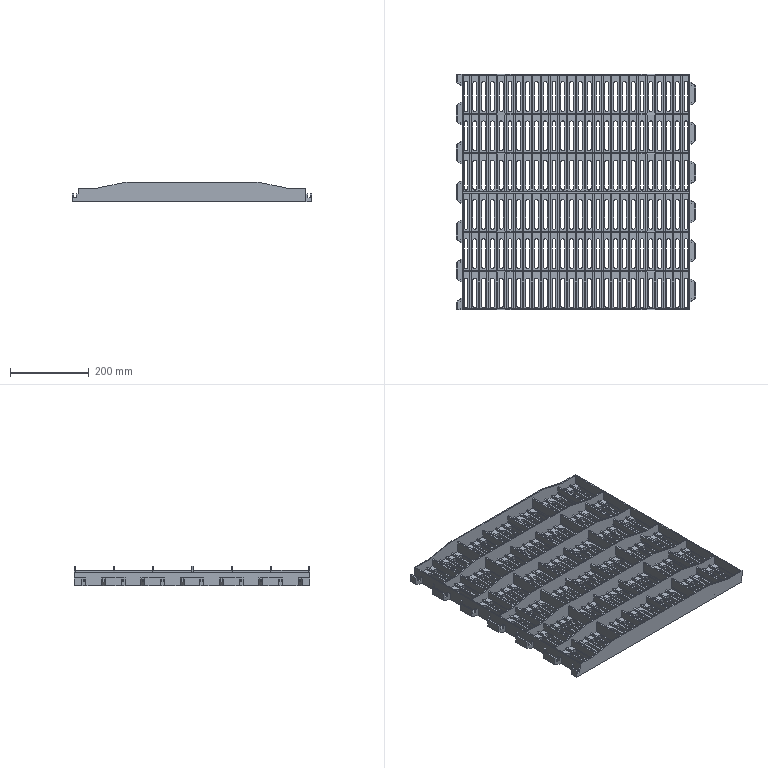Part | SolidWorks | features ICE 7, LPattern 4, MirrorPattern 4, BossThin 1, Extrusion 1 | 1 solid | 1519 faces | box 610 x 600 x 50 mm | volume 3519467 mm3 | plane 1193 | cylinder 326 | commonest cylinder face diameters 10 x312 100 x14